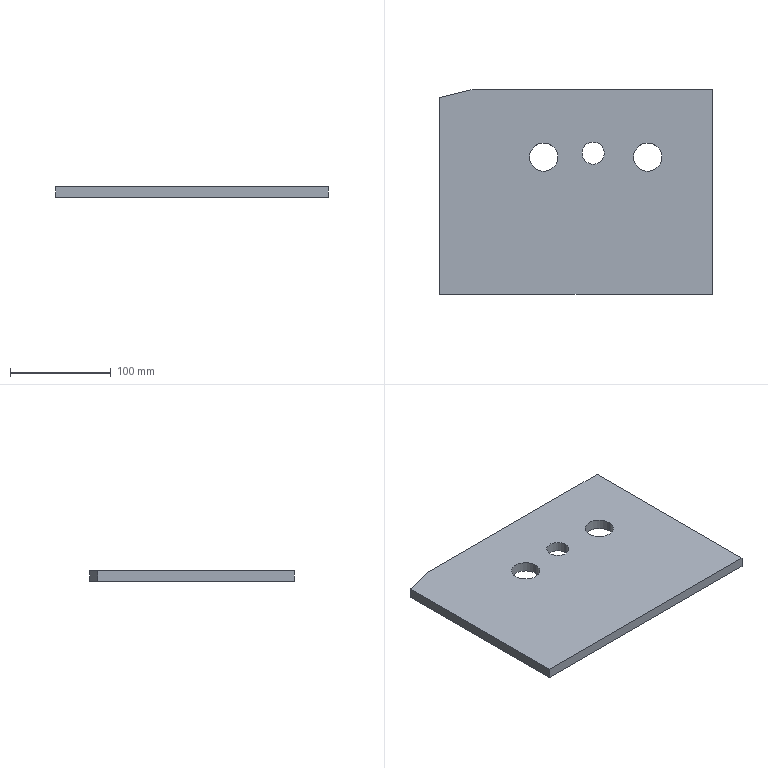Part | STEP file | 001-003-Shaft storage magazine adjusting plate | 1 solid | 13 faces | box 270 x 203 x 10 mm | volume 530707 mm3 | plane 7 | cylinder 6 | commonest cylinder face diameters 28 x4 22 x2
STEP:
#1=CARTESIAN_POINT('',(0.,0.,0.));
#2=DIRECTION('',(0.,0.,1.));
#3=DIRECTION('',(1.,0.,0.));
#4=AXIS2_PLACEMENT_3D('',#1,#2,#3);
#5=CARTESIAN_POINT('',(-18.,34.5,0.));
#6=VERTEX_POINT('',#5);
#7=CARTESIAN_POINT('',(-18.,34.5,10.));
#8=VERTEX_POINT('',#7);
#9=CARTESIAN_POINT('',(-18.,34.5,0.));
#10=DIRECTION('',(0.,0.,1.));
#11=VECTOR('',#10,1.);
#12=LINE('',#9,#11);
#13=CARTESIAN_POINT('',(-32.,34.5,0.));
#14=DIRECTION('',(0.,0.,1.));
#15=DIRECTION('',(1.,0.,0.));
#16=AXIS2_PLACEMENT_3D('',#13,#14,#15);
#17=CYLINDRICAL_SURFACE('',#16,14.);
#18=CARTESIAN_POINT('',(6.283,0.));
#19=DIRECTION('',(0.,1.));
#20=VECTOR('',#19,1.);
#21=LINE('',#18,#20);
#22=(GEOMETRIC_REPRESENTATION_CONTEXT(2)PARAMETRIC_REPRESENTATION_CONTEXT()REPRESENTATION_CONTEXT('',''));
#23=DEFINITIONAL_REPRESENTATION('',(#21),#22);
#24=PCURVE('',#17,#23);
#25=CARTESIAN_POINT('',(-32.,34.5,0.));
#26=DIRECTION('',(0.,0.,1.));
#27=DIRECTION('',(1.,0.,0.));
#28=AXIS2_PLACEMENT_3D('',#25,#26,#27);
#29=CYLINDRICAL_SURFACE('',#28,14.);
#30=CARTESIAN_POINT('',(0.,0.));
#31=DIRECTION('',(0.,1.));
#32=VECTOR('',#31,1.);
#33=LINE('',#30,#32);
#34=(GEOMETRIC_REPRESENTATION_CONTEXT(2)PARAMETRIC_REPRESENTATION_CONTEXT()REPRESENTATION_CONTEXT('',''));
#35=DEFINITIONAL_REPRESENTATION('',(#33),#34);
#36=PCURVE('',#29,#35);
#37=SURFACE_CURVE('',#12,(#24,#36),.PCURVE_S1.);
#38=EDGE_CURVE('',#6,#8,#37,.T.);
#39=ORIENTED_EDGE('',*,*,#38,.T.);
#40=CARTESIAN_POINT('',(-46.,34.5,10.));
#41=VERTEX_POINT('',#40);
#42=CARTESIAN_POINT('',(-32.,34.5,10.));
#43=DIRECTION('',(0.,0.,1.));
#44=DIRECTION('',(1.,0.,0.));
#45=AXIS2_PLACEMENT_3D('',#42,#43,#44);
#46=CIRCLE('',#45,14.);
#47=CARTESIAN_POINT('',(0.,10.));
#48=DIRECTION('',(1.,0.));
#49=VECTOR('',#48,1.);
#50=LINE('',#47,#49);
#51=(GEOMETRIC_REPRESENTATION_CONTEXT(2)PARAMETRIC_REPRESENTATION_CONTEXT()REPRESENTATION_CONTEXT('',''));
#52=DEFINITIONAL_REPRESENTATION('',(#50),#51);
#53=PCURVE('',#17,#52);
#54=CARTESIAN_POINT('',(0.,0.,10.));
#55=DIRECTION('',(0.,0.,-1.));
#56=DIRECTION('',(-1.,0.,0.));
#57=AXIS2_PLACEMENT_3D('',#54,#55,#56);
#58=PLANE('',#57);
#59=CARTESIAN_POINT('',(18.,34.5));
#60=CARTESIAN_POINT('',(18.,58.749));
#61=CARTESIAN_POINT('',(39.,46.624));
#62=CARTESIAN_POINT('',(60.,34.5));
#63=CARTESIAN_POINT('',(39.,22.376));
#64=CARTESIAN_POINT('',(18.,10.251));
#65=CARTESIAN_POINT('',(18.,34.5));
#66=(BOUNDED_CURVE()B_SPLINE_CURVE(2,(#59,#60,#61,#62,#63,#64,#65),.UNSPECIFIED.,.T.,.F.)B_SPLINE_CURVE_WITH_KNOTS((1,2,2,2,2,1),(-2.094,0.,2.094,4.189,6.283,8.378),.UNSPECIFIED.)CURVE()GEOMETRIC_REPRESENTATION_ITEM()RATIONAL_B_SPLINE_CURVE((1.,0.5,1.,0.5,1.,0.5,1.))REPRESENTATION_ITEM(''));
#67=(GEOMETRIC_REPRESENTATION_CONTEXT(2)PARAMETRIC_REPRESENTATION_CONTEXT()REPRESENTATION_CONTEXT('',''));
#68=DEFINITIONAL_REPRESENTATION('',(#66),#67);
#69=PCURVE('',#58,#68);
#70=SURFACE_CURVE('',#46,(#53,#69),.PCURVE_S1.);
#71=EDGE_CURVE('',#41,#8,#70,.T.);
#72=ORIENTED_EDGE('',*,*,#71,.F.);
#73=CARTESIAN_POINT('',(-46.,34.5,0.));
#74=VERTEX_POINT('',#73);
#75=CARTESIAN_POINT('',(-46.,34.5,0.));
#76=DIRECTION('',(0.,0.,1.));
#77=VECTOR('',#76,1.);
#78=LINE('',#75,#77);
#79=CARTESIAN_POINT('',(3.142,0.));
#80=DIRECTION('',(0.,1.));
#81=VECTOR('',#80,1.);
#82=LINE('',#79,#81);
#83=(GEOMETRIC_REPRESENTATION_CONTEXT(2)PARAMETRIC_REPRESENTATION_CONTEXT()REPRESENTATION_CONTEXT('',''));
#84=DEFINITIONAL_REPRESENTATION('',(#82),#83);
#85=PCURVE('',#17,#84);
#86=CARTESIAN_POINT('',(3.142,0.));
#87=DIRECTION('',(0.,1.));
#88=VECTOR('',#87,1.);
#89=LINE('',#86,#88);
#90=(GEOMETRIC_REPRESENTATION_CONTEXT(2)PARAMETRIC_REPRESENTATION_CONTEXT()REPRESENTATION_CONTEXT('',''));
#91=DEFINITIONAL_REPRESENTATION('',(#89),#90);
#92=PCURVE('',#29,#91);
#93=SURFACE_CURVE('',#78,(#85,#92),.PCURVE_S1.);
#94=EDGE_CURVE('',#74,#41,#93,.T.);
#95=ORIENTED_EDGE('',*,*,#94,.F.);
#96=CARTESIAN_POINT('',(-32.,34.5,0.));
#97=DIRECTION('',(0.,0.,1.));
#98=DIRECTION('',(1.,0.,0.));
#99=AXIS2_PLACEMENT_3D('',#96,#97,#98);
#100=CIRCLE('',#99,14.);
#101=CARTESIAN_POINT('',(0.,0.));
#102=DIRECTION('',(1.,0.));
#103=VECTOR('',#102,1.);
#104=LINE('',#101,#103);
#105=(GEOMETRIC_REPRESENTATION_CONTEXT(2)PARAMETRIC_REPRESENTATION_CONTEXT()REPRESENTATION_CONTEXT('',''));
#106=DEFINITIONAL_REPRESENTATION('',(#104),#105);
#107=PCURVE('',#17,#106);
#108=CARTESIAN_POINT('',(0.,0.,0.));
#109=DIRECTION('',(0.,0.,-1.));
#110=DIRECTION('',(-1.,0.,0.));
#111=AXIS2_PLACEMENT_3D('',#108,#109,#110);
#112=PLANE('',#111);
#113=CARTESIAN_POINT('',(18.,34.5));
#114=CARTESIAN_POINT('',(18.,58.749));
#115=CARTESIAN_POINT('',(39.,46.624));
#116=CARTESIAN_POINT('',(60.,34.5));
#117=CARTESIAN_POINT('',(39.,22.376));
#118=CARTESIAN_POINT('',(18.,10.251));
#119=CARTESIAN_POINT('',(18.,34.5));
#120=(BOUNDED_CURVE()B_SPLINE_CURVE(2,(#113,#114,#115,#116,#117,#118,#119),.UNSPECIFIED.,.T.,.F.)B_SPLINE_CURVE_WITH_KNOTS((1,2,2,2,2,1),(-2.094,0.,2.094,4.189,6.283,8.378),.UNSPECIFIED.)CURVE()GEOMETRIC_REPRESENTATION_ITEM()RATIONAL_B_SPLINE_CURVE((1.,0.5,1.,0.5,1.,0.5,1.))REPRESENTATION_ITEM(''));
#121=(GEOMETRIC_REPRESENTATION_CONTEXT(2)PARAMETRIC_REPRESENTATION_CONTEXT()REPRESENTATION_CONTEXT('',''));
#122=DEFINITIONAL_REPRESENTATION('',(#120),#121);
#123=PCURVE('',#112,#122);
#124=SURFACE_CURVE('',#100,(#107,#123),.PCURVE_S1.);
#125=EDGE_CURVE('',#74,#6,#124,.T.);
#126=ORIENTED_EDGE('',*,*,#125,.T.);
#127=EDGE_LOOP('',(#39,#72,#95,#126));
#128=FACE_BOUND('',#127,.F.);
#129=ADVANCED_FACE('',(#128),#17,.F.);
#130=CARTESIAN_POINT('',(85.,34.5,0.));
#131=VERTEX_POINT('',#130);
#132=CARTESIAN_POINT('',(85.,34.5,10.));
#133=VERTEX_POINT('',#132);
#134=CARTESIAN_POINT('',(85.,34.5,0.));
#135=DIRECTION('',(0.,0.,1.));
#136=VECTOR('',#135,1.);
#137=LINE('',#134,#136);
#138=CARTESIAN_POINT('',(71.,34.5,0.));
#139=DIRECTION('',(0.,0.,1.));
#140=DIRECTION('',(1.,0.,0.));
#141=AXIS2_PLACEMENT_3D('',#138,#139,#140);
#142=CYLINDRICAL_SURFACE('',#141,14.);
#143=CARTESIAN_POINT('',(6.283,0.));
#144=DIRECTION('',(0.,1.));
#145=VECTOR('',#144,1.);
#146=LINE('',#143,#145);
#147=(GEOMETRIC_REPRESENTATION_CONTEXT(2)PARAMETRIC_REPRESENTATION_CONTEXT()REPRESENTATION_CONTEXT('',''));
#148=DEFINITIONAL_REPRESENTATION('',(#146),#147);
#149=PCURVE('',#142,#148);
#150=CARTESIAN_POINT('',(71.,34.5,0.));
#151=DIRECTION('',(0.,0.,1.));
#152=DIRECTION('',(1.,0.,0.));
#153=AXIS2_PLACEMENT_3D('',#150,#151,#152);
#154=CYLINDRICAL_SURFACE('',#153,14.);
#155=CARTESIAN_POINT('',(0.,0.));
#156=DIRECTION('',(0.,1.));
#157=VECTOR('',#156,1.);
#158=LINE('',#155,#157);
#159=(GEOMETRIC_REPRESENTATION_CONTEXT(2)PARAMETRIC_REPRESENTATION_CONTEXT()REPRESENTATION_CONTEXT('',''));
#160=DEFINITIONAL_REPRESENTATION('',(#158),#159);
#161=PCURVE('',#154,#160);
#162=SURFACE_CURVE('',#137,(#149,#161),.PCURVE_S1.);
#163=EDGE_CURVE('',#131,#133,#162,.T.);
#164=ORIENTED_EDGE('',*,*,#163,.T.);
#165=CARTESIAN_POINT('',(57.,34.5,10.));
#166=VERTEX_POINT('',#165);
#167=CARTESIAN_POINT('',(71.,34.5,10.));
#168=DIRECTION('',(0.,0.,1.));
#169=DIRECTION('',(1.,0.,0.));
#170=AXIS2_PLACEMENT_3D('',#167,#168,#169);
#171=CIRCLE('',#170,14.);
#172=CARTESIAN_POINT('',(0.,10.));
#173=DIRECTION('',(1.,0.));
#174=VECTOR('',#173,1.);
#175=LINE('',#172,#174);
#176=(GEOMETRIC_REPRESENTATION_CONTEXT(2)PARAMETRIC_REPRESENTATION_CONTEXT()REPRESENTATION_CONTEXT('',''));
#177=DEFINITIONAL_REPRESENTATION('',(#175),#176);
#178=PCURVE('',#142,#177);
#179=CARTESIAN_POINT('',(-85.,34.5));
#180=CARTESIAN_POINT('',(-85.,58.749));
#181=CARTESIAN_POINT('',(-64.,46.624));
#182=CARTESIAN_POINT('',(-43.,34.5));
#183=CARTESIAN_POINT('',(-64.,22.376));
#184=CARTESIAN_POINT('',(-85.,10.251));
#185=CARTESIAN_POINT('',(-85.,34.5));
#186=(BOUNDED_CURVE()B_SPLINE_CURVE(2,(#179,#180,#181,#182,#183,#184,#185),.UNSPECIFIED.,.T.,.F.)B_SPLINE_CURVE_WITH_KNOTS((1,2,2,2,2,1),(-2.094,0.,2.094,4.189,6.283,8.378),.UNSPECIFIED.)CURVE()GEOMETRIC_REPRESENTATION_ITEM()RATIONAL_B_SPLINE_CURVE((1.,0.5,1.,0.5,1.,0.5,1.))REPRESENTATION_ITEM(''));
#187=(GEOMETRIC_REPRESENTATION_CONTEXT(2)PARAMETRIC_REPRESENTATION_CONTEXT()REPRESENTATION_CONTEXT('',''));
#188=DEFINITIONAL_REPRESENTATION('',(#186),#187);
#189=PCURVE('',#58,#188);
#190=SURFACE_CURVE('',#171,(#178,#189),.PCURVE_S1.);
#191=EDGE_CURVE('',#166,#133,#190,.T.);
#192=ORIENTED_EDGE('',*,*,#191,.F.);
#193=CARTESIAN_POINT('',(57.,34.5,0.));
#194=VERTEX_POINT('',#193);
#195=CARTESIAN_POINT('',(57.,34.5,0.));
#196=DIRECTION('',(0.,0.,1.));
#197=VECTOR('',#196,1.);
#198=LINE('',#195,#197);
#199=CARTESIAN_POINT('',(3.142,0.));
#200=DIRECTION('',(0.,1.));
#201=VECTOR('',#200,1.);
#202=LINE('',#199,#201);
#203=(GEOMETRIC_REPRESENTATION_CONTEXT(2)PARAMETRIC_REPRESENTATION_CONTEXT()REPRESENTATION_CONTEXT('',''));
#204=DEFINITIONAL_REPRESENTATION('',(#202),#203);
#205=PCURVE('',#142,#204);
#206=CARTESIAN_POINT('',(3.142,0.));
#207=DIRECTION('',(0.,1.));
#208=VECTOR('',#207,1.);
#209=LINE('',#206,#208);
#210=(GEOMETRIC_REPRESENTATION_CONTEXT(2)PARAMETRIC_REPRESENTATION_CONTEXT()REPRESENTATION_CONTEXT('',''));
#211=DEFINITIONAL_REPRESENTATION('',(#209),#210);
#212=PCURVE('',#154,#211);
#213=SURFACE_CURVE('',#198,(#205,#212),.PCURVE_S1.);
#214=EDGE_CURVE('',#194,#166,#213,.T.);
#215=ORIENTED_EDGE('',*,*,#214,.F.);
#216=CARTESIAN_POINT('',(71.,34.5,0.));
#217=DIRECTION('',(0.,0.,1.));
#218=DIRECTION('',(1.,0.,0.));
#219=AXIS2_PLACEMENT_3D('',#216,#217,#218);
#220=CIRCLE('',#219,14.);
#221=CARTESIAN_POINT('',(0.,0.));
#222=DIRECTION('',(1.,0.));
#223=VECTOR('',#222,1.);
#224=LINE('',#221,#223);
#225=(GEOMETRIC_REPRESENTATION_CONTEXT(2)PARAMETRIC_REPRESENTATION_CONTEXT()REPRESENTATION_CONTEXT('',''));
#226=DEFINITIONAL_REPRESENTATION('',(#224),#225);
#227=PCURVE('',#142,#226);
#228=CARTESIAN_POINT('',(-85.,34.5));
#229=CARTESIAN_POINT('',(-85.,58.749));
#230=CARTESIAN_POINT('',(-64.,46.624));
#231=CARTESIAN_POINT('',(-43.,34.5));
#232=CARTESIAN_POINT('',(-64.,22.376));
#233=CARTESIAN_POINT('',(-85.,10.251));
#234=CARTESIAN_POINT('',(-85.,34.5));
#235=(BOUNDED_CURVE()B_SPLINE_CURVE(2,(#228,#229,#230,#231,#232,#233,#234),.UNSPECIFIED.,.T.,.F.)B_SPLINE_CURVE_WITH_KNOTS((1,2,2,2,2,1),(-2.094,0.,2.094,4.189,6.283,8.378),.UNSPECIFIED.)CURVE()GEOMETRIC_REPRESENTATION_ITEM()RATIONAL_B_SPLINE_CURVE((1.,0.5,1.,0.5,1.,0.5,1.))REPRESENTATION_ITEM(''));
#236=(GEOMETRIC_REPRESENTATION_CONTEXT(2)PARAMETRIC_REPRESENTATION_CONTEXT()REPRESENTATION_CONTEXT('',''));
#237=DEFINITIONAL_REPRESENTATION('',(#235),#236);
#238=PCURVE('',#112,#237);
#239=SURFACE_CURVE('',#220,(#227,#238),.PCURVE_S1.);
#240=EDGE_CURVE('',#194,#131,#239,.T.);
#241=ORIENTED_EDGE('',*,*,#240,.T.);
#242=EDGE_LOOP('',(#164,#192,#215,#241));
#243=FACE_BOUND('',#242,.F.);
#244=ADVANCED_FACE('',(#243),#142,.F.);
#245=CARTESIAN_POINT('',(28.,38.5,0.));
#246=VERTEX_POINT('',#245);
#247=CARTESIAN_POINT('',(28.,38.5,10.));
#248=VERTEX_POINT('',#247);
#249=CARTESIAN_POINT('',(28.,38.5,0.));
#250=DIRECTION('',(0.,0.,1.));
#251=VECTOR('',#250,1.);
#252=LINE('',#249,#251);
#253=CARTESIAN_POINT('',(17.,38.5,0.));
#254=DIRECTION('',(0.,0.,1.));
#255=DIRECTION('',(1.,0.,0.));
#256=AXIS2_PLACEMENT_3D('',#253,#254,#255);
#257=CYLINDRICAL_SURFACE('',#256,11.);
#258=CARTESIAN_POINT('',(6.283,0.));
#259=DIRECTION('',(0.,1.));
#260=VECTOR('',#259,1.);
#261=LINE('',#258,#260);
#262=(GEOMETRIC_REPRESENTATION_CONTEXT(2)PARAMETRIC_REPRESENTATION_CONTEXT()REPRESENTATION_CONTEXT('',''));
#263=DEFINITIONAL_REPRESENTATION('',(#261),#262);
#264=PCURVE('',#257,#263);
#265=CARTESIAN_POINT('',(17.,38.5,0.));
#266=DIRECTION('',(0.,0.,1.));
#267=DIRECTION('',(1.,0.,0.));
#268=AXIS2_PLACEMENT_3D('',#265,#266,#267);
#269=CYLINDRICAL_SURFACE('',#268,11.);
#270=CARTESIAN_POINT('',(0.,0.));
#271=DIRECTION('',(0.,1.));
#272=VECTOR('',#271,1.);
#273=LINE('',#270,#272);
#274=(GEOMETRIC_REPRESENTATION_CONTEXT(2)PARAMETRIC_REPRESENTATION_CONTEXT()REPRESENTATION_CONTEXT('',''));
#275=DEFINITIONAL_REPRESENTATION('',(#273),#274);
#276=PCURVE('',#269,#275);
#277=SURFACE_CURVE('',#252,(#264,#276),.PCURVE_S1.);
#278=EDGE_CURVE('',#246,#248,#277,.T.);
#279=ORIENTED_EDGE('',*,*,#278,.T.);
#280=CARTESIAN_POINT('',(6.,38.5,10.));
#281=VERTEX_POINT('',#280);
#282=CARTESIAN_POINT('',(17.,38.5,10.));
#283=DIRECTION('',(0.,0.,1.));
#284=DIRECTION('',(1.,0.,0.));
#285=AXIS2_PLACEMENT_3D('',#282,#283,#284);
#286=CIRCLE('',#285,11.);
#287=CARTESIAN_POINT('',(0.,10.));
#288=DIRECTION('',(1.,0.));
#289=VECTOR('',#288,1.);
#290=LINE('',#287,#289);
#291=(GEOMETRIC_REPRESENTATION_CONTEXT(2)PARAMETRIC_REPRESENTATION_CONTEXT()REPRESENTATION_CONTEXT('',''));
#292=DEFINITIONAL_REPRESENTATION('',(#290),#291);
#293=PCURVE('',#257,#292);
#294=CARTESIAN_POINT('',(-28.,38.5));
#295=CARTESIAN_POINT('',(-28.,57.553));
#296=CARTESIAN_POINT('',(-11.5,48.026));
#297=CARTESIAN_POINT('',(5.,38.5));
#298=CARTESIAN_POINT('',(-11.5,28.974));
#299=CARTESIAN_POINT('',(-28.,19.447));
#300=CARTESIAN_POINT('',(-28.,38.5));
#301=(BOUNDED_CURVE()B_SPLINE_CURVE(2,(#294,#295,#296,#297,#298,#299,#300),.UNSPECIFIED.,.T.,.F.)B_SPLINE_CURVE_WITH_KNOTS((1,2,2,2,2,1),(-2.094,0.,2.094,4.189,6.283,8.378),.UNSPECIFIED.)CURVE()GEOMETRIC_REPRESENTATION_ITEM()RATIONAL_B_SPLINE_CURVE((1.,0.5,1.,0.5,1.,0.5,1.))REPRESENTATION_ITEM(''));
#302=(GEOMETRIC_REPRESENTATION_CONTEXT(2)PARAMETRIC_REPRESENTATION_CONTEXT()REPRESENTATION_CONTEXT('',''));
#303=DEFINITIONAL_REPRESENTATION('',(#301),#302);
#304=PCURVE('',#58,#303);
#305=SURFACE_CURVE('',#286,(#293,#304),.PCURVE_S1.);
#306=EDGE_CURVE('',#281,#248,#305,.T.);
#307=ORIENTED_EDGE('',*,*,#306,.F.);
#308=CARTESIAN_POINT('',(6.,38.5,0.));
#309=VERTEX_POINT('',#308);
#310=CARTESIAN_POINT('',(6.,38.5,0.));
#311=DIRECTION('',(0.,0.,1.));
#312=VECTOR('',#311,1.);
#313=LINE('',#310,#312);
#314=CARTESIAN_POINT('',(3.142,0.));
#315=DIRECTION('',(0.,1.));
#316=VECTOR('',#315,1.);
#317=LINE('',#314,#316);
#318=(GEOMETRIC_REPRESENTATION_CONTEXT(2)PARAMETRIC_REPRESENTATION_CONTEXT()REPRESENTATION_CONTEXT('',''));
#319=DEFINITIONAL_REPRESENTATION('',(#317),#318);
#320=PCURVE('',#257,#319);
#321=CARTESIAN_POINT('',(3.142,0.));
#322=DIRECTION('',(0.,1.));
#323=VECTOR('',#322,1.);
#324=LINE('',#321,#323);
#325=(GEOMETRIC_REPRESENTATION_CONTEXT(2)PARAMETRIC_REPRESENTATION_CONTEXT()REPRESENTATION_CONTEXT('',''));
#326=DEFINITIONAL_REPRESENTATION('',(#324),#325);
#327=PCURVE('',#269,#326);
#328=SURFACE_CURVE('',#313,(#320,#327),.PCURVE_S1.);
#329=EDGE_CURVE('',#309,#281,#328,.T.);
#330=ORIENTED_EDGE('',*,*,#329,.F.);
#331=CARTESIAN_POINT('',(17.,38.5,0.));
#332=DIRECTION('',(0.,0.,1.));
#333=DIRECTION('',(1.,0.,0.));
#334=AXIS2_PLACEMENT_3D('',#331,#332,#333);
#335=CIRCLE('',#334,11.);
#336=CARTESIAN_POINT('',(0.,0.));
#337=DIRECTION('',(1.,0.));
#338=VECTOR('',#337,1.);
#339=LINE('',#336,#338);
#340=(GEOMETRIC_REPRESENTATION_CONTEXT(2)PARAMETRIC_REPRESENTATION_CONTEXT()REPRESENTATION_CONTEXT('',''));
#341=DEFINITIONAL_REPRESENTATION('',(#339),#340);
#342=PCURVE('',#257,#341);
#343=CARTESIAN_POINT('',(-28.,38.5));
#344=CARTESIAN_POINT('',(-28.,57.553));
#345=CARTESIAN_POINT('',(-11.5,48.026));
#346=CARTESIAN_POINT('',(5.,38.5));
#347=CARTESIAN_POINT('',(-11.5,28.974));
#348=CARTESIAN_POINT('',(-28.,19.447));
#349=CARTESIAN_POINT('',(-28.,38.5));
#350=(BOUNDED_CURVE()B_SPLINE_CURVE(2,(#343,#344,#345,#346,#347,#348,#349),.UNSPECIFIED.,.T.,.F.)B_SPLINE_CURVE_WITH_KNOTS((1,2,2,2,2,1),(-2.094,0.,2.094,4.189,6.283,8.378),.UNSPECIFIED.)CURVE()GEOMETRIC_REPRESENTATION_ITEM()RATIONAL_B_SPLINE_CURVE((1.,0.5,1.,0.5,1.,0.5,1.))REPRESENTATION_ITEM(''));
#351=(GEOMETRIC_REPRESENTATION_CONTEXT(2)PARAMETRIC_REPRESENTATION_CONTEXT()REPRESENTATION_CONTEXT('',''));
#352=DEFINITIONAL_REPRESENTATION('',(#350),#351);
#353=PCURVE('',#112,#352);
#354=SURFACE_CURVE('',#335,(#342,#353),.PCURVE_S1.);
#355=EDGE_CURVE('',#309,#246,#354,.T.);
#356=ORIENTED_EDGE('',*,*,#355,.T.);
#357=EDGE_LOOP('',(#279,#307,#330,#356));
#358=FACE_BOUND('',#357,.F.);
#359=ADVANCED_FACE('',(#358),#257,.F.);
#360=CARTESIAN_POINT('',(-103.,101.5,10.));
#361=VERTEX_POINT('',#360);
#362=CARTESIAN_POINT('',(-103.,101.5,0.));
#363=VERTEX_POINT('',#362);
#364=CARTESIAN_POINT('',(-103.,101.5,10.));
#365=DIRECTION('',(0.,0.,-1.));
#366=VECTOR('',#365,1.);
#367=LINE('',#364,#366);
#368=CARTESIAN_POINT('',(-135.,101.5,10.));
#369=DIRECTION('',(0.,-1.,0.));
#370=DIRECTION('',(0.,0.,-1.));
#371=AXIS2_PLACEMENT_3D('',#368,#369,#370);
#372=PLANE('',#371);
#373=CARTESIAN_POINT('',(0.,32.));
#374=DIRECTION('',(1.,0.));
#375=VECTOR('',#374,1.);
#376=LINE('',#373,#375);
#377=(GEOMETRIC_REPRESENTATION_CONTEXT(2)PARAMETRIC_REPRESENTATION_CONTEXT()REPRESENTATION_CONTEXT('',''));
#378=DEFINITIONAL_REPRESENTATION('',(#376),#377);
#379=PCURVE('',#372,#378);
#380=CARTESIAN_POINT('',(-103.,101.5,10.));
#381=DIRECTION('',(-0.2419,0.9703,0.));
#382=DIRECTION('',(-0.9703,-0.2419,0.));
#383=AXIS2_PLACEMENT_3D('',#380,#381,#382);
#384=PLANE('',#383);
#385=CARTESIAN_POINT('',(0.,0.));
#386=DIRECTION('',(0.,-1.));
#387=VECTOR('',#386,1.);
#388=LINE('',#385,#387);
#389=(GEOMETRIC_REPRESENTATION_CONTEXT(2)PARAMETRIC_REPRESENTATION_CONTEXT()REPRESENTATION_CONTEXT('',''));
#390=DEFINITIONAL_REPRESENTATION('',(#388),#389);
#391=PCURVE('',#384,#390);
#392=SURFACE_CURVE('',#367,(#379,#391),.PCURVE_S1.);
#393=EDGE_CURVE('',#361,#363,#392,.T.);
#394=ORIENTED_EDGE('',*,*,#393,.F.);
#395=CARTESIAN_POINT('',(135.,101.5,10.));
#396=VERTEX_POINT('',#395);
#397=CARTESIAN_POINT('',(-135.,101.5,10.));
#398=DIRECTION('',(-1.,0.,0.));
#399=VECTOR('',#398,1.);
#400=LINE('',#397,#399);
#401=CARTESIAN_POINT('',(0.,0.));
#402=DIRECTION('',(0.,-1.));
#403=VECTOR('',#402,1.);
#404=LINE('',#401,#403);
#405=(GEOMETRIC_REPRESENTATION_CONTEXT(2)PARAMETRIC_REPRESENTATION_CONTEXT()REPRESENTATION_CONTEXT('',''));
#406=DEFINITIONAL_REPRESENTATION('',(#404),#405);
#407=PCURVE('',#372,#406);
#408=CARTESIAN_POINT('',(135.,101.5));
#409=DIRECTION('',(1.,0.));
#410=VECTOR('',#409,1.);
#411=LINE('',#408,#410);
#412=(GEOMETRIC_REPRESENTATION_CONTEXT(2)PARAMETRIC_REPRESENTATION_CONTEXT()REPRESENTATION_CONTEXT('',''));
#413=DEFINITIONAL_REPRESENTATION('',(#411),#412);
#414=PCURVE('',#58,#413);
#415=SURFACE_CURVE('',#400,(#407,#414),.PCURVE_S1.);
#416=EDGE_CURVE('',#396,#361,#415,.T.);
#417=ORIENTED_EDGE('',*,*,#416,.F.);
#418=CARTESIAN_POINT('',(135.,101.5,0.));
#419=VERTEX_POINT('',#418);
#420=CARTESIAN_POINT('',(135.,101.5,10.));
#421=DIRECTION('',(0.,0.,-1.));
#422=VECTOR('',#421,1.);
#423=LINE('',#420,#422);
#424=CARTESIAN_POINT('',(0.,270.));
#425=DIRECTION('',(1.,0.));
#426=VECTOR('',#425,1.);
#427=LINE('',#424,#426);
#428=(GEOMETRIC_REPRESENTATION_CONTEXT(2)PARAMETRIC_REPRESENTATION_CONTEXT()REPRESENTATION_CONTEXT('',''));
#429=DEFINITIONAL_REPRESENTATION('',(#427),#428);
#430=PCURVE('',#372,#429);
#431=CARTESIAN_POINT('',(135.,-101.5,10.));
#432=DIRECTION('',(-1.,0.,0.));
#433=DIRECTION('',(0.,0.,1.));
#434=AXIS2_PLACEMENT_3D('',#431,#432,#433);
#435=PLANE('',#434);
#436=CARTESIAN_POINT('',(0.,203.));
#437=DIRECTION('',(-1.,0.));
#438=VECTOR('',#437,1.);
#439=LINE('',#436,#438);
#440=(GEOMETRIC_REPRESENTATION_CONTEXT(2)PARAMETRIC_REPRESENTATION_CONTEXT()REPRESENTATION_CONTEXT('',''));
#441=DEFINITIONAL_REPRESENTATION('',(#439),#440);
#442=PCURVE('',#435,#441);
#443=SURFACE_CURVE('',#423,(#430,#442),.PCURVE_S1.);
#444=EDGE_CURVE('',#396,#419,#443,.T.);
#445=ORIENTED_EDGE('',*,*,#444,.T.);
#446=CARTESIAN_POINT('',(-135.,101.5,0.));
#447=DIRECTION('',(-1.,0.,0.));
#448=VECTOR('',#447,1.);
#449=LINE('',#446,#448);
#450=CARTESIAN_POINT('',(10.,0.));
#451=DIRECTION('',(0.,-1.));
#452=VECTOR('',#451,1.);
#453=LINE('',#450,#452);
#454=(GEOMETRIC_REPRESENTATION_CONTEXT(2)PARAMETRIC_REPRESENTATION_CONTEXT()REPRESENTATION_CONTEXT('',''));
#455=DEFINITIONAL_REPRESENTATION('',(#453),#454);
#456=PCURVE('',#372,#455);
#457=CARTESIAN_POINT('',(135.,101.5));
#458=DIRECTION('',(1.,0.));
#459=VECTOR('',#458,1.);
#460=LINE('',#457,#459);
#461=(GEOMETRIC_REPRESENTATION_CONTEXT(2)PARAMETRIC_REPRESENTATION_CONTEXT()REPRESENTATION_CONTEXT('',''));
#462=DEFINITIONAL_REPRESENTATION('',(#460),#461);
#463=PCURVE('',#112,#462);
#464=SURFACE_CURVE('',#449,(#456,#463),.PCURVE_S1.);
#465=EDGE_CURVE('',#419,#363,#464,.T.);
#466=ORIENTED_EDGE('',*,*,#465,.T.);
#467=EDGE_LOOP('',(#394,#417,#445,#466));
#468=FACE_BOUND('',#467,.T.);
#469=ADVANCED_FACE('',(#468),#372,.F.);
#470=CARTESIAN_POINT('',(-135.,93.522,10.));
#471=VERTEX_POINT('',#470);
#472=CARTESIAN_POINT('',(-135.,93.522,0.));
#473=VERTEX_POINT('',#472);
#474=CARTESIAN_POINT('',(-135.,93.522,10.));
#475=DIRECTION('',(0.,0.,-1.));
#476=VECTOR('',#475,1.);
#477=LINE('',#474,#476);
#478=CARTESIAN_POINT('',(-135.,-101.5,10.));
#479=DIRECTION('',(1.,0.,0.));
#480=DIRECTION('',(0.,0.,-1.));
#481=AXIS2_PLACEMENT_3D('',#478,#479,#480);
#482=PLANE('',#481);
#483=CARTESIAN_POINT('',(0.,195.022));
#484=DIRECTION('',(1.,0.));
#485=VECTOR('',#484,1.);
#486=LINE('',#483,#485);
#487=(GEOMETRIC_REPRESENTATION_CONTEXT(2)PARAMETRIC_REPRESENTATION_CONTEXT()REPRESENTATION_CONTEXT('',''));
#488=DEFINITIONAL_REPRESENTATION('',(#486),#487);
#489=PCURVE('',#482,#488);
#490=CARTESIAN_POINT('',(32.98,0.));
#491=DIRECTION('',(0.,-1.));
#492=VECTOR('',#491,1.);
#493=LINE('',#490,#492);
#494=(GEOMETRIC_REPRESENTATION_CONTEXT(2)PARAMETRIC_REPRESENTATION_CONTEXT()REPRESENTATION_CONTEXT('',''));
#495=DEFINITIONAL_REPRESENTATION('',(#493),#494);
#496=PCURVE('',#384,#495);
#497=SURFACE_CURVE('',#477,(#489,#496),.PCURVE_S1.);
#498=EDGE_CURVE('',#471,#473,#497,.T.);
#499=ORIENTED_EDGE('',*,*,#498,.T.);
#500=CARTESIAN_POINT('',(-135.,-101.5,0.));
#501=VERTEX_POINT('',#500);
#502=CARTESIAN_POINT('',(-135.,-101.5,0.));
#503=DIRECTION('',(0.,-1.,0.));
#504=VECTOR('',#503,1.);
#505=LINE('',#502,#504);
#506=CARTESIAN_POINT('',(10.,0.));
#507=DIRECTION('',(0.,-1.));
#508=VECTOR('',#507,1.);
#509=LINE('',#506,#508);
#510=(GEOMETRIC_REPRESENTATION_CONTEXT(2)PARAMETRIC_REPRESENTATION_CONTEXT()REPRESENTATION_CONTEXT('',''));
#511=DEFINITIONAL_REPRESENTATION('',(#509),#510);
#512=PCURVE('',#482,#511);
#513=CARTESIAN_POINT('',(135.,-101.5));
#514=DIRECTION('',(0.,-1.));
#515=VECTOR('',#514,1.);
#516=LINE('',#513,#515);
#517=(GEOMETRIC_REPRESENTATION_CONTEXT(2)PARAMETRIC_REPRESENTATION_CONTEXT()REPRESENTATION_CONTEXT('',''));
#518=DEFINITIONAL_REPRESENTATION('',(#516),#517);
#519=PCURVE('',#112,#518);
#520=SURFACE_CURVE('',#505,(#512,#519),.PCURVE_S1.);
#521=EDGE_CURVE('',#473,#501,#520,.T.);
#522=ORIENTED_EDGE('',*,*,#521,.T.);
#523=CARTESIAN_POINT('',(-135.,-101.5,10.));
#524=VERTEX_POINT('',#523);
#525=CARTESIAN_POINT('',(-135.,-101.5,10.));
#526=DIRECTION('',(0.,0.,-1.));
#527=VECTOR('',#526,1.);
#528=LINE('',#525,#527);
#529=CARTESIAN_POINT('',(0.,0.));
#530=DIRECTION('',(1.,0.));
#531=VECTOR('',#530,1.);
#532=LINE('',#529,#531);
#533=(GEOMETRIC_REPRESENTATION_CONTEXT(2)PARAMETRIC_REPRESENTATION_CONTEXT()REPRESENTATION_CONTEXT('',''));
#534=DEFINITIONAL_REPRESENTATION('',(#532),#533);
#535=PCURVE('',#482,#534);
#536=CARTESIAN_POINT('',(-135.,-101.5,10.));
#537=DIRECTION('',(0.,1.,0.));
#538=DIRECTION('',(0.,0.,1.));
#539=AXIS2_PLACEMENT_3D('',#536,#537,#538);
#540=PLANE('',#539);
#541=CARTESIAN_POINT('',(0.,0.));
#542=DIRECTION('',(-1.,0.));
#543=VECTOR('',#542,1.);
#544=LINE('',#541,#543);
#545=(GEOMETRIC_REPRESENTATION_CONTEXT(2)PARAMETRIC_REPRESENTATION_CONTEXT()REPRESENTATION_CONTEXT('',''));
#546=DEFINITIONAL_REPRESENTATION('',(#544),#545);
#547=PCURVE('',#540,#546);
#548=SURFACE_CURVE('',#528,(#535,#547),.PCURVE_S1.);
#549=EDGE_CURVE('',#524,#501,#548,.T.);
#550=ORIENTED_EDGE('',*,*,#549,.F.);
#551=CARTESIAN_POINT('',(-135.,-101.5,10.));
#552=DIRECTION('',(0.,-1.,0.));
#553=VECTOR('',#552,1.);
#554=LINE('',#551,#553);
#555=CARTESIAN_POINT('',(0.,0.));
#556=DIRECTION('',(0.,-1.));
#557=VECTOR('',#556,1.);
#558=LINE('',#555,#557);
#559=(GEOMETRIC_REPRESENTATION_CONTEXT(2)PARAMETRIC_REPRESENTATION_CONTEXT()REPRESENTATION_CONTEXT('',''));
#560=DEFINITIONAL_REPRESENTATION('',(#558),#559);
#561=PCURVE('',#482,#560);
#562=CARTESIAN_POINT('',(135.,-101.5));
#563=DIRECTION('',(0.,-1.));
#564=VECTOR('',#563,1.);
#565=LINE('',#562,#564);
#566=(GEOMETRIC_REPRESENTATION_CONTEXT(2)PARAMETRIC_REPRESENTATION_CONTEXT()REPRESENTATION_CONTEXT('',''));
#567=DEFINITIONAL_REPRESENTATION('',(#565),#566);
#568=PCURVE('',#58,#567);
#569=SURFACE_CURVE('',#554,(#561,#568),.PCURVE_S1.);
#570=EDGE_CURVE('',#471,#524,#569,.T.);
#571=ORIENTED_EDGE('',*,*,#570,.F.);
#572=EDGE_LOOP('',(#499,#522,#550,#571));
#573=FACE_BOUND('',#572,.T.);
#574=ADVANCED_FACE('',(#573),#482,.F.);
#575=CARTESIAN_POINT('',(-32.,34.5,10.));
#576=DIRECTION('',(0.,0.,1.));
#577=DIRECTION('',(1.,0.,0.));
#578=AXIS2_PLACEMENT_3D('',#575,#576,#577);
#579=CIRCLE('',#578,14.);
#580=CARTESIAN_POINT('',(18.,34.5));
#581=CARTESIAN_POINT('',(18.,58.749));
#582=CARTESIAN_POINT('',(39.,46.624));
#583=CARTESIAN_POINT('',(60.,34.5));
#584=CARTESIAN_POINT('',(39.,22.376));
#585=CARTESIAN_POINT('',(18.,10.251));
#586=CARTESIAN_POINT('',(18.,34.5));
#587=(BOUNDED_CURVE()B_SPLINE_CURVE(2,(#580,#581,#582,#583,#584,#585,#586),.UNSPECIFIED.,.T.,.F.)B_SPLINE_CURVE_WITH_KNOTS((1,2,2,2,2,1),(-2.094,0.,2.094,4.189,6.283,8.378),.UNSPECIFIED.)CURVE()GEOMETRIC_REPRESENTATION_ITEM()RATIONAL_B_SPLINE_CURVE((1.,0.5,1.,0.5,1.,0.5,1.))REPRESENTATION_ITEM(''));
#588=(GEOMETRIC_REPRESENTATION_CONTEXT(2)PARAMETRIC_REPRESENTATION_CONTEXT()REPRESENTATION_CONTEXT('',''));
#589=DEFINITIONAL_REPRESENTATION('',(#587),#588);
#590=PCURVE('',#58,#589);
#591=CARTESIAN_POINT('',(0.,10.));
#592=DIRECTION('',(1.,0.));
#593=VECTOR('',#592,1.);
#594=LINE('',#591,#593);
#595=(GEOMETRIC_REPRESENTATION_CONTEXT(2)PARAMETRIC_REPRESENTATION_CONTEXT()REPRESENTATION_CONTEXT('',''));
#596=DEFINITIONAL_REPRESENTATION('',(#594),#595);
#597=PCURVE('',#29,#596);
#598=SURFACE_CURVE('',#579,(#590,#597),.PCURVE_S1.);
#599=EDGE_CURVE('',#8,#41,#598,.T.);
#600=ORIENTED_EDGE('',*,*,#599,.F.);
#601=ORIENTED_EDGE('',*,*,#71,.F.);
#602=EDGE_LOOP('',(#600,#601));
#603=FACE_BOUND('',#602,.T.);
#604=CARTESIAN_POINT('',(71.,34.5,10.));
#605=DIRECTION('',(0.,0.,1.));
#606=DIRECTION('',(1.,0.,0.));
#607=AXIS2_PLACEMENT_3D('',#604,#605,#606);
#608=CIRCLE('',#607,14.);
#609=CARTESIAN_POINT('',(-85.,34.5));
#610=CARTESIAN_POINT('',(-85.,58.749));
#611=CARTESIAN_POINT('',(-64.,46.624));
#612=CARTESIAN_POINT('',(-43.,34.5));
#613=CARTESIAN_POINT('',(-64.,22.376));
#614=CARTESIAN_POINT('',(-85.,10.251));
#615=CARTESIAN_POINT('',(-85.,34.5));
#616=(BOUNDED_CURVE()B_SPLINE_CURVE(2,(#609,#610,#611,#612,#613,#614,#615),.UNSPECIFIED.,.T.,.F.)B_SPLINE_CURVE_WITH_KNOTS((1,2,2,2,2,1),(-2.094,0.,2.094,4.189,6.283,8.378),.UNSPECIFIED.)CURVE()GEOMETRIC_REPRESENTATION_ITEM()RATIONAL_B_SPLINE_CURVE((1.,0.5,1.,0.5,1.,0.5,1.))REPRESENTATION_ITEM(''));
#617=(GEOMETRIC_REPRESENTATION_CONTEXT(2)PARAMETRIC_REPRESENTATION_CONTEXT()REPRESENTATION_CONTEXT('',''));
#618=DEFINITIONAL_REPRESENTATION('',(#616),#617);
#619=PCURVE('',#58,#618);
#620=CARTESIAN_POINT('',(0.,10.));
#621=DIRECTION('',(1.,0.));
#622=VECTOR('',#621,1.);
#623=LINE('',#620,#622);
#624=(GEOMETRIC_REPRESENTATION_CONTEXT(2)PARAMETRIC_REPRESENTATION_CONTEXT()REPRESENTATION_CONTEXT('',''));
#625=DEFINITIONAL_REPRESENTATION('',(#623),#624);
#626=PCURVE('',#154,#625);
#627=SURFACE_CURVE('',#608,(#619,#626),.PCURVE_S1.);
#628=EDGE_CURVE('',#133,#166,#627,.T.);
#629=ORIENTED_EDGE('',*,*,#628,.F.);
#630=ORIENTED_EDGE('',*,*,#191,.F.);
#631=EDGE_LOOP('',(#629,#630));
#632=FACE_BOUND('',#631,.T.);
#633=CARTESIAN_POINT('',(17.,38.5,10.));
#634=DIRECTION('',(0.,0.,1.));
#635=DIRECTION('',(1.,0.,0.));
#636=AXIS2_PLACEMENT_3D('',#633,#634,#635);
#637=CIRCLE('',#636,11.);
#638=CARTESIAN_POINT('',(-28.,38.5));
#639=CARTESIAN_POINT('',(-28.,57.553));
#640=CARTESIAN_POINT('',(-11.5,48.026));
#641=CARTESIAN_POINT('',(5.,38.5));
#642=CARTESIAN_POINT('',(-11.5,28.974));
#643=CARTESIAN_POINT('',(-28.,19.447));
#644=CARTESIAN_POINT('',(-28.,38.5));
#645=(BOUNDED_CURVE()B_SPLINE_CURVE(2,(#638,#639,#640,#641,#642,#643,#644),.UNSPECIFIED.,.T.,.F.)B_SPLINE_CURVE_WITH_KNOTS((1,2,2,2,2,1),(-2.094,0.,2.094,4.189,6.283,8.378),.UNSPECIFIED.)CURVE()GEOMETRIC_REPRESENTATION_ITEM()RATIONAL_B_SPLINE_CURVE((1.,0.5,1.,0.5,1.,0.5,1.))REPRESENTATION_ITEM(''));
#646=(GEOMETRIC_REPRESENTATION_CONTEXT(2)PARAMETRIC_REPRESENTATION_CONTEXT()REPRESENTATION_CONTEXT('',''));
#647=DEFINITIONAL_REPRESENTATION('',(#645),#646);
#648=PCURVE('',#58,#647);
#649=CARTESIAN_POINT('',(0.,10.));
#650=DIRECTION('',(1.,0.));
#651=VECTOR('',#650,1.);
#652=LINE('',#649,#651);
#653=(GEOMETRIC_REPRESENTATION_CONTEXT(2)PARAMETRIC_REPRESENTATION_CONTEXT()REPRESENTATION_CONTEXT('',''));
#654=DEFINITIONAL_REPRESENTATION('',(#652),#653);
#655=PCURVE('',#269,#654);
#656=SURFACE_CURVE('',#637,(#648,#655),.PCURVE_S1.);
#657=EDGE_CURVE('',#248,#281,#656,.T.);
#658=ORIENTED_EDGE('',*,*,#657,.F.);
#659=ORIENTED_EDGE('',*,*,#306,.F.);
#660=EDGE_LOOP('',(#658,#659));
#661=FACE_BOUND('',#660,.T.);
#662=CARTESIAN_POINT('',(-103.,101.5,10.));
#663=DIRECTION('',(0.9703,0.2419,0.));
#664=VECTOR('',#663,1.);
#665=LINE('',#662,#664);
#666=CARTESIAN_POINT('',(103.,101.5));
#667=DIRECTION('',(-0.9703,0.2419));
#668=VECTOR('',#667,1.);
#669=LINE('',#666,#668);
#670=(GEOMETRIC_REPRESENTATION_CONTEXT(2)PARAMETRIC_REPRESENTATION_CONTEXT()REPRESENTATION_CONTEXT('',''));
#671=DEFINITIONAL_REPRESENTATION('',(#669),#670);
#672=PCURVE('',#58,#671);
#673=CARTESIAN_POINT('',(0.,0.));
#674=DIRECTION('',(-1.,0.));
#675=VECTOR('',#674,1.);
#676=LINE('',#673,#675);
#677=(GEOMETRIC_REPRESENTATION_CONTEXT(2)PARAMETRIC_REPRESENTATION_CONTEXT()REPRESENTATION_CONTEXT('',''));
#678=DEFINITIONAL_REPRESENTATION('',(#676),#677);
#679=PCURVE('',#384,#678);
#680=SURFACE_CURVE('',#665,(#672,#679),.PCURVE_S1.);
#681=EDGE_CURVE('',#471,#361,#680,.T.);
#682=ORIENTED_EDGE('',*,*,#681,.F.);
#683=ORIENTED_EDGE('',*,*,#570,.T.);
#684=CARTESIAN_POINT('',(135.,-101.5,10.));
#685=VERTEX_POINT('',#684);
#686=CARTESIAN_POINT('',(-135.,-101.5,10.));
#687=DIRECTION('',(1.,0.,0.));
#688=VECTOR('',#687,1.);
#689=LINE('',#686,#688);
#690=CARTESIAN_POINT('',(135.,-101.5));
#691=DIRECTION('',(-1.,0.));
#692=VECTOR('',#691,1.);
#693=LINE('',#690,#692);
#694=(GEOMETRIC_REPRESENTATION_CONTEXT(2)PARAMETRIC_REPRESENTATION_CONTEXT()REPRESENTATION_CONTEXT('',''));
#695=DEFINITIONAL_REPRESENTATION('',(#693),#694);
#696=PCURVE('',#58,#695);
#697=CARTESIAN_POINT('',(0.,0.));
#698=DIRECTION('',(0.,1.));
#699=VECTOR('',#698,1.);
#700=LINE('',#697,#699);
#701=(GEOMETRIC_REPRESENTATION_CONTEXT(2)PARAMETRIC_REPRESENTATION_CONTEXT()REPRESENTATION_CONTEXT('',''));
#702=DEFINITIONAL_REPRESENTATION('',(#700),#701);
#703=PCURVE('',#540,#702);
#704=SURFACE_CURVE('',#689,(#696,#703),.PCURVE_S1.);
#705=EDGE_CURVE('',#524,#685,#704,.T.);
#706=ORIENTED_EDGE('',*,*,#705,.T.);
#707=CARTESIAN_POINT('',(135.,-101.5,10.));
#708=DIRECTION('',(0.,1.,0.));
#709=VECTOR('',#708,1.);
#710=LINE('',#707,#709);
#711=CARTESIAN_POINT('',(-135.,-101.5));
#712=DIRECTION('',(0.,1.));
#713=VECTOR('',#712,1.);
#714=LINE('',#711,#713);
#715=(GEOMETRIC_REPRESENTATION_CONTEXT(2)PARAMETRIC_REPRESENTATION_CONTEXT()REPRESENTATION_CONTEXT('',''));
#716=DEFINITIONAL_REPRESENTATION('',(#714),#715);
#717=PCURVE('',#58,#716);
#718=CARTESIAN_POINT('',(0.,0.));
#719=DIRECTION('',(0.,1.));
#720=VECTOR('',#719,1.);
#721=LINE('',#718,#720);
#722=(GEOMETRIC_REPRESENTATION_CONTEXT(2)PARAMETRIC_REPRESENTATION_CONTEXT()REPRESENTATION_CONTEXT('',''));
#723=DEFINITIONAL_REPRESENTATION('',(#721),#722);
#724=PCURVE('',#435,#723);
#725=SURFACE_CURVE('',#710,(#717,#724),.PCURVE_S1.);
#726=EDGE_CURVE('',#685,#396,#725,.T.);
#727=ORIENTED_EDGE('',*,*,#726,.T.);
#728=ORIENTED_EDGE('',*,*,#416,.T.);
#729=EDGE_LOOP('',(#682,#683,#706,#727,#728));
#730=FACE_BOUND('',#729,.T.);
#731=ADVANCED_FACE('',(#603,#632,#661,#730),#58,.F.);
#732=CARTESIAN_POINT('',(-32.,34.5,0.));
#733=DIRECTION('',(0.,0.,1.));
#734=DIRECTION('',(1.,0.,0.));
#735=AXIS2_PLACEMENT_3D('',#732,#733,#734);
#736=CIRCLE('',#735,14.);
#737=CARTESIAN_POINT('',(18.,34.5));
#738=CARTESIAN_POINT('',(18.,58.749));
#739=CARTESIAN_POINT('',(39.,46.624));
#740=CARTESIAN_POINT('',(60.,34.5));
#741=CARTESIAN_POINT('',(39.,22.376));
#742=CARTESIAN_POINT('',(18.,10.251));
#743=CARTESIAN_POINT('',(18.,34.5));
#744=(BOUNDED_CURVE()B_SPLINE_CURVE(2,(#737,#738,#739,#740,#741,#742,#743),.UNSPECIFIED.,.T.,.F.)B_SPLINE_CURVE_WITH_KNOTS((1,2,2,2,2,1),(-2.094,0.,2.094,4.189,6.283,8.378),.UNSPECIFIED.)CURVE()GEOMETRIC_REPRESENTATION_ITEM()RATIONAL_B_SPLINE_CURVE((1.,0.5,1.,0.5,1.,0.5,1.))REPRESENTATION_ITEM(''));
#745=(GEOMETRIC_REPRESENTATION_CONTEXT(2)PARAMETRIC_REPRESENTATION_CONTEXT()REPRESENTATION_CONTEXT('',''));
#746=DEFINITIONAL_REPRESENTATION('',(#744),#745);
#747=PCURVE('',#112,#746);
#748=CARTESIAN_POINT('',(0.,0.));
#749=DIRECTION('',(1.,0.));
#750=VECTOR('',#749,1.);
#751=LINE('',#748,#750);
#752=(GEOMETRIC_REPRESENTATION_CONTEXT(2)PARAMETRIC_REPRESENTATION_CONTEXT()REPRESENTATION_CONTEXT('',''));
#753=DEFINITIONAL_REPRESENTATION('',(#751),#752);
#754=PCURVE('',#29,#753);
#755=SURFACE_CURVE('',#736,(#747,#754),.PCURVE_S1.);
#756=EDGE_CURVE('',#6,#74,#755,.T.);
#757=ORIENTED_EDGE('',*,*,#756,.T.);
#758=ORIENTED_EDGE('',*,*,#125,.T.);
#759=EDGE_LOOP('',(#757,#758));
#760=FACE_BOUND('',#759,.T.);
#761=CARTESIAN_POINT('',(71.,34.5,0.));
#762=DIRECTION('',(0.,0.,1.));
#763=DIRECTION('',(1.,0.,0.));
#764=AXIS2_PLACEMENT_3D('',#761,#762,#763);
#765=CIRCLE('',#764,14.);
#766=CARTESIAN_POINT('',(-85.,34.5));
#767=CARTESIAN_POINT('',(-85.,58.749));
#768=CARTESIAN_POINT('',(-64.,46.624));
#769=CARTESIAN_POINT('',(-43.,34.5));
#770=CARTESIAN_POINT('',(-64.,22.376));
#771=CARTESIAN_POINT('',(-85.,10.251));
#772=CARTESIAN_POINT('',(-85.,34.5));
#773=(BOUNDED_CURVE()B_SPLINE_CURVE(2,(#766,#767,#768,#769,#770,#771,#772),.UNSPECIFIED.,.T.,.F.)B_SPLINE_CURVE_WITH_KNOTS((1,2,2,2,2,1),(-2.094,0.,2.094,4.189,6.283,8.378),.UNSPECIFIED.)CURVE()GEOMETRIC_REPRESENTATION_ITEM()RATIONAL_B_SPLINE_CURVE((1.,0.5,1.,0.5,1.,0.5,1.))REPRESENTATION_ITEM(''));
#774=(GEOMETRIC_REPRESENTATION_CONTEXT(2)PARAMETRIC_REPRESENTATION_CONTEXT()REPRESENTATION_CONTEXT('',''));
#775=DEFINITIONAL_REPRESENTATION('',(#773),#774);
#776=PCURVE('',#112,#775);
#777=CARTESIAN_POINT('',(0.,0.));
#778=DIRECTION('',(1.,0.));
#779=VECTOR('',#778,1.);
#780=LINE('',#777,#779);
#781=(GEOMETRIC_REPRESENTATION_CONTEXT(2)PARAMETRIC_REPRESENTATION_CONTEXT()REPRESENTATION_CONTEXT('',''));
#782=DEFINITIONAL_REPRESENTATION('',(#780),#781);
#783=PCURVE('',#154,#782);
#784=SURFACE_CURVE('',#765,(#776,#783),.PCURVE_S1.);
#785=EDGE_CURVE('',#131,#194,#784,.T.);
#786=ORIENTED_EDGE('',*,*,#785,.T.);
#787=ORIENTED_EDGE('',*,*,#240,.T.);
#788=EDGE_LOOP('',(#786,#787));
#789=FACE_BOUND('',#788,.T.);
#790=CARTESIAN_POINT('',(17.,38.5,0.));
#791=DIRECTION('',(0.,0.,1.));
#792=DIRECTION('',(1.,0.,0.));
#793=AXIS2_PLACEMENT_3D('',#790,#791,#792);
#794=CIRCLE('',#793,11.);
#795=CARTESIAN_POINT('',(-28.,38.5));
#796=CARTESIAN_POINT('',(-28.,57.553));
#797=CARTESIAN_POINT('',(-11.5,48.026));
#798=CARTESIAN_POINT('',(5.,38.5));
#799=CARTESIAN_POINT('',(-11.5,28.974));
#800=CARTESIAN_POINT('',(-28.,19.447));
#801=CARTESIAN_POINT('',(-28.,38.5));
#802=(BOUNDED_CURVE()B_SPLINE_CURVE(2,(#795,#796,#797,#798,#799,#800,#801),.UNSPECIFIED.,.T.,.F.)B_SPLINE_CURVE_WITH_KNOTS((1,2,2,2,2,1),(-2.094,0.,2.094,4.189,6.283,8.378),.UNSPECIFIED.)CURVE()GEOMETRIC_REPRESENTATION_ITEM()RATIONAL_B_SPLINE_CURVE((1.,0.5,1.,0.5,1.,0.5,1.))REPRESENTATION_ITEM(''));
#803=(GEOMETRIC_REPRESENTATION_CONTEXT(2)PARAMETRIC_REPRESENTATION_CONTEXT()REPRESENTATION_CONTEXT('',''));
#804=DEFINITIONAL_REPRESENTATION('',(#802),#803);
#805=PCURVE('',#112,#804);
#806=CARTESIAN_POINT('',(0.,0.));
#807=DIRECTION('',(1.,0.));
#808=VECTOR('',#807,1.);
#809=LINE('',#806,#808);
#810=(GEOMETRIC_REPRESENTATION_CONTEXT(2)PARAMETRIC_REPRESENTATION_CONTEXT()REPRESENTATION_CONTEXT('',''));
#811=DEFINITIONAL_REPRESENTATION('',(#809),#810);
#812=PCURVE('',#269,#811);
#813=SURFACE_CURVE('',#794,(#805,#812),.PCURVE_S1.);
#814=EDGE_CURVE('',#246,#309,#813,.T.);
#815=ORIENTED_EDGE('',*,*,#814,.T.);
#816=ORIENTED_EDGE('',*,*,#355,.T.);
#817=EDGE_LOOP('',(#815,#816));
#818=FACE_BOUND('',#817,.T.);
#819=ORIENTED_EDGE('',*,*,#521,.F.);
#820=CARTESIAN_POINT('',(-103.,101.5,0.));
#821=DIRECTION('',(0.9703,0.2419,0.));
#822=VECTOR('',#821,1.);
#823=LINE('',#820,#822);
#824=CARTESIAN_POINT('',(103.,101.5));
#825=DIRECTION('',(-0.9703,0.2419));
#826=VECTOR('',#825,1.);
#827=LINE('',#824,#826);
#828=(GEOMETRIC_REPRESENTATION_CONTEXT(2)PARAMETRIC_REPRESENTATION_CONTEXT()REPRESENTATION_CONTEXT('',''));
#829=DEFINITIONAL_REPRESENTATION('',(#827),#828);
#830=PCURVE('',#112,#829);
#831=CARTESIAN_POINT('',(0.,-10.));
#832=DIRECTION('',(-1.,0.));
#833=VECTOR('',#832,1.);
#834=LINE('',#831,#833);
#835=(GEOMETRIC_REPRESENTATION_CONTEXT(2)PARAMETRIC_REPRESENTATION_CONTEXT()REPRESENTATION_CONTEXT('',''));
#836=DEFINITIONAL_REPRESENTATION('',(#834),#835);
#837=PCURVE('',#384,#836);
#838=SURFACE_CURVE('',#823,(#830,#837),.PCURVE_S1.);
#839=EDGE_CURVE('',#473,#363,#838,.T.);
#840=ORIENTED_EDGE('',*,*,#839,.T.);
#841=ORIENTED_EDGE('',*,*,#465,.F.);
#842=CARTESIAN_POINT('',(135.,-101.5,0.));
#843=VERTEX_POINT('',#842);
#844=CARTESIAN_POINT('',(135.,-101.5,0.));
#845=DIRECTION('',(0.,1.,0.));
#846=VECTOR('',#845,1.);
#847=LINE('',#844,#846);
#848=CARTESIAN_POINT('',(-135.,-101.5));
#849=DIRECTION('',(0.,1.));
#850=VECTOR('',#849,1.);
#851=LINE('',#848,#850);
#852=(GEOMETRIC_REPRESENTATION_CONTEXT(2)PARAMETRIC_REPRESENTATION_CONTEXT()REPRESENTATION_CONTEXT('',''));
#853=DEFINITIONAL_REPRESENTATION('',(#851),#852);
#854=PCURVE('',#112,#853);
#855=CARTESIAN_POINT('',(-10.,0.));
#856=DIRECTION('',(0.,1.));
#857=VECTOR('',#856,1.);
#858=LINE('',#855,#857);
#859=(GEOMETRIC_REPRESENTATION_CONTEXT(2)PARAMETRIC_REPRESENTATION_CONTEXT()REPRESENTATION_CONTEXT('',''));
#860=DEFINITIONAL_REPRESENTATION('',(#858),#859);
#861=PCURVE('',#435,#860);
#862=SURFACE_CURVE('',#847,(#854,#861),.PCURVE_S1.);
#863=EDGE_CURVE('',#843,#419,#862,.T.);
#864=ORIENTED_EDGE('',*,*,#863,.F.);
#865=CARTESIAN_POINT('',(-135.,-101.5,0.));
#866=DIRECTION('',(1.,0.,0.));
#867=VECTOR('',#866,1.);
#868=LINE('',#865,#867);
#869=CARTESIAN_POINT('',(135.,-101.5));
#870=DIRECTION('',(-1.,0.));
#871=VECTOR('',#870,1.);
#872=LINE('',#869,#871);
#873=(GEOMETRIC_REPRESENTATION_CONTEXT(2)PARAMETRIC_REPRESENTATION_CONTEXT()REPRESENTATION_CONTEXT('',''));
#874=DEFINITIONAL_REPRESENTATION('',(#872),#873);
#875=PCURVE('',#112,#874);
#876=CARTESIAN_POINT('',(-10.,0.));
#877=DIRECTION('',(0.,1.));
#878=VECTOR('',#877,1.);
#879=LINE('',#876,#878);
#880=(GEOMETRIC_REPRESENTATION_CONTEXT(2)PARAMETRIC_REPRESENTATION_CONTEXT()REPRESENTATION_CONTEXT('',''));
#881=DEFINITIONAL_REPRESENTATION('',(#879),#880);
#882=PCURVE('',#540,#881);
#883=SURFACE_CURVE('',#868,(#875,#882),.PCURVE_S1.);
#884=EDGE_CURVE('',#501,#843,#883,.T.);
#885=ORIENTED_EDGE('',*,*,#884,.F.);
#886=EDGE_LOOP('',(#819,#840,#841,#864,#885));
#887=FACE_BOUND('',#886,.T.);
#888=ADVANCED_FACE('',(#760,#789,#818,#887),#112,.T.);
#889=ORIENTED_EDGE('',*,*,#863,.T.);
#890=ORIENTED_EDGE('',*,*,#444,.F.);
#891=ORIENTED_EDGE('',*,*,#726,.F.);
#892=CARTESIAN_POINT('',(135.,-101.5,10.));
#893=DIRECTION('',(0.,0.,-1.));
#894=VECTOR('',#893,1.);
#895=LINE('',#892,#894);
#896=CARTESIAN_POINT('',(0.,0.));
#897=DIRECTION('',(-1.,0.));
#898=VECTOR('',#897,1.);
#899=LINE('',#896,#898);
#900=(GEOMETRIC_REPRESENTATION_CONTEXT(2)PARAMETRIC_REPRESENTATION_CONTEXT()REPRESENTATION_CONTEXT('',''));
#901=DEFINITIONAL_REPRESENTATION('',(#899),#900);
#902=PCURVE('',#435,#901);
#903=CARTESIAN_POINT('',(0.,270.));
#904=DIRECTION('',(-1.,0.));
#905=VECTOR('',#904,1.);
#906=LINE('',#903,#905);
#907=(GEOMETRIC_REPRESENTATION_CONTEXT(2)PARAMETRIC_REPRESENTATION_CONTEXT()REPRESENTATION_CONTEXT('',''));
#908=DEFINITIONAL_REPRESENTATION('',(#906),#907);
#909=PCURVE('',#540,#908);
#910=SURFACE_CURVE('',#895,(#902,#909),.PCURVE_S1.);
#911=EDGE_CURVE('',#685,#843,#910,.T.);
#912=ORIENTED_EDGE('',*,*,#911,.T.);
#913=EDGE_LOOP('',(#889,#890,#891,#912));
#914=FACE_BOUND('',#913,.T.);
#915=ADVANCED_FACE('',(#914),#435,.F.);
#916=ORIENTED_EDGE('',*,*,#884,.T.);
#917=ORIENTED_EDGE('',*,*,#911,.F.);
#918=ORIENTED_EDGE('',*,*,#705,.F.);
#919=ORIENTED_EDGE('',*,*,#549,.T.);
#920=EDGE_LOOP('',(#916,#917,#918,#919));
#921=FACE_BOUND('',#920,.T.);
#922=ADVANCED_FACE('',(#921),#540,.F.);
#923=ORIENTED_EDGE('',*,*,#839,.F.);
#924=ORIENTED_EDGE('',*,*,#498,.F.);
#925=ORIENTED_EDGE('',*,*,#681,.T.);
#926=ORIENTED_EDGE('',*,*,#393,.T.);
#927=EDGE_LOOP('',(#923,#924,#925,#926));
#928=FACE_BOUND('',#927,.T.);
#929=ADVANCED_FACE('',(#928),#384,.T.);
#930=ORIENTED_EDGE('',*,*,#657,.F.);
#931=ORIENTED_EDGE('',*,*,#278,.F.);
#932=ORIENTED_EDGE('',*,*,#814,.T.);
#933=ORIENTED_EDGE('',*,*,#329,.T.);
#934=EDGE_LOOP('',(#930,#931,#932,#933));
#935=FACE_BOUND('',#934,.F.);
#936=ADVANCED_FACE('',(#935),#269,.F.);
#937=ORIENTED_EDGE('',*,*,#628,.F.);
#938=ORIENTED_EDGE('',*,*,#163,.F.);
#939=ORIENTED_EDGE('',*,*,#785,.T.);
#940=ORIENTED_EDGE('',*,*,#214,.T.);
#941=EDGE_LOOP('',(#937,#938,#939,#940));
#942=FACE_BOUND('',#941,.F.);
#943=ADVANCED_FACE('',(#942),#154,.F.);
#944=ORIENTED_EDGE('',*,*,#599,.F.);
#945=ORIENTED_EDGE('',*,*,#38,.F.);
#946=ORIENTED_EDGE('',*,*,#756,.T.);
#947=ORIENTED_EDGE('',*,*,#94,.T.);
#948=EDGE_LOOP('',(#944,#945,#946,#947));
#949=FACE_BOUND('',#948,.F.);
#950=ADVANCED_FACE('',(#949),#29,.F.);
#951=CLOSED_SHELL('',(#129,#244,#359,#469,#574,#731,#888,#915,#922,#929,#936,#943,#950));
#952=MANIFOLD_SOLID_BREP('',#951);
#953=(LENGTH_UNIT()NAMED_UNIT(*)SI_UNIT(.MILLI.,.METRE.));
#954=UNCERTAINTY_MEASURE_WITH_UNIT(LENGTH_MEASURE(0.0000001),#953,'','');
#955=(NAMED_UNIT(*)PLANE_ANGLE_UNIT()SI_UNIT($,.RADIAN.));
#956=(NAMED_UNIT(*)SI_UNIT($,.STERADIAN.)SOLID_ANGLE_UNIT());
#957=(GEOMETRIC_REPRESENTATION_CONTEXT(3)GLOBAL_UNCERTAINTY_ASSIGNED_CONTEXT((#954))GLOBAL_UNIT_ASSIGNED_CONTEXT((#953,#955,#956))REPRESENTATION_CONTEXT('',''));
#958=ADVANCED_BREP_SHAPE_REPRESENTATION('',(#4,#952),#957);